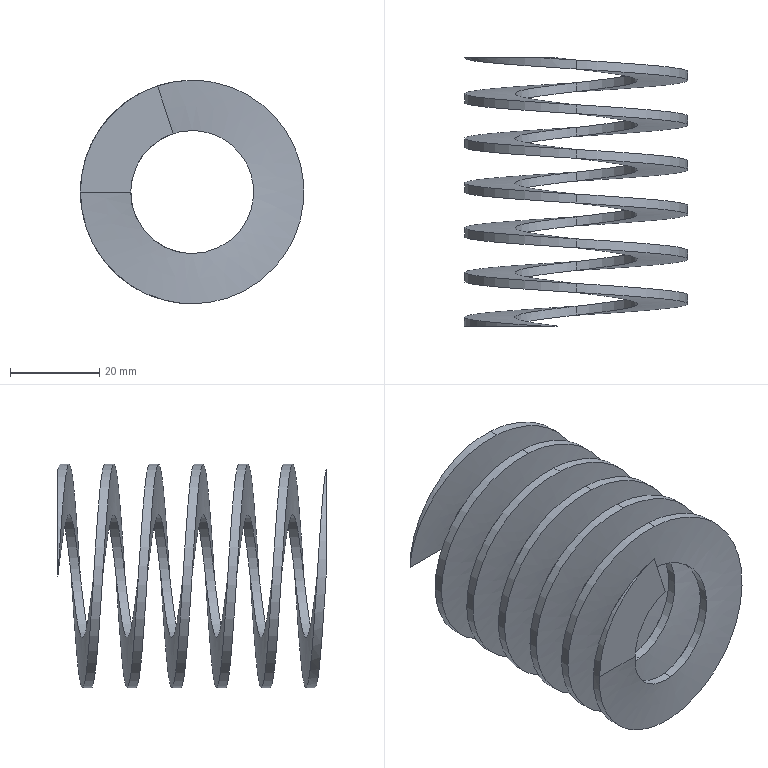Part | STEP file | PN_0023_default | 1 solid | 30 faces | box 50 x 60 x 50 mm | volume 16434 mm3 | cylinder 26 | spline 2 | plane 2 | commonest cylinder face diameters 27.5 x13 50 x13